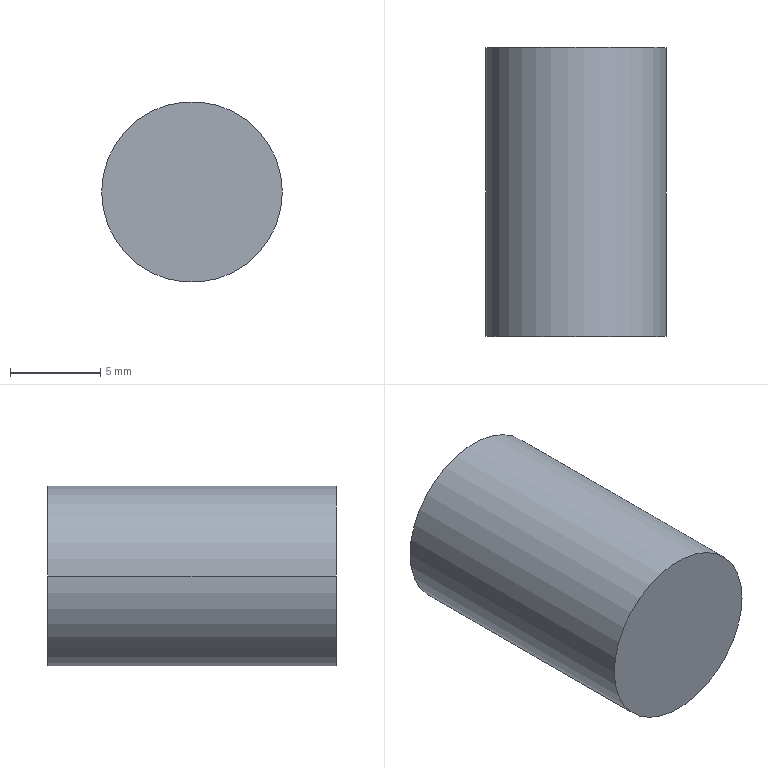Part | SolidWorks | features Chamfer 1, ICE 1, Revolution 1 | 1 solid | 9 faces | box 10 x 16 x 10 mm | volume 971.407 mm3 | cylinder 4 | plane 3 | cone 2 | commonest cylinder face diameters 6 x2 10 x2
STEP:
#1=CARTESIAN_POINT('',(3.,-0.5,0.));
#2=VERTEX_POINT('',#1);
#3=CARTESIAN_POINT('',(-3.,-0.5,0.));
#4=VERTEX_POINT('',#3);
#5=CARTESIAN_POINT('',(0.,-0.5,0.));
#6=DIRECTION('',(0.,1.,0.));
#7=DIRECTION('',(-1.,0.,0.));
#8=AXIS2_PLACEMENT_3D('',#5,#6,#7);
#9=CIRCLE('',#8,3.);
#10=EDGE_CURVE('',#2,#4,#9,.T.);
#11=ORIENTED_EDGE('',*,*,#10,.F.);
#12=CARTESIAN_POINT('',(3.5,0.,0.));
#13=VERTEX_POINT('',#12);
#14=CARTESIAN_POINT('',(3.,-0.5,0.));
#15=DIRECTION('',(0.7071,0.7071,0.));
#16=VECTOR('',#15,1000.);
#17=LINE('',#14,#16);
#18=EDGE_CURVE('',#2,#13,#17,.T.);
#19=ORIENTED_EDGE('',*,*,#18,.T.);
#20=CARTESIAN_POINT('',(-3.5,0.,0.));
#21=VERTEX_POINT('',#20);
#22=CARTESIAN_POINT('',(0.,0.,0.));
#23=DIRECTION('',(0.,-1.,0.));
#24=DIRECTION('',(-1.,0.,0.));
#25=AXIS2_PLACEMENT_3D('',#22,#23,#24);
#26=CIRCLE('',#25,3.5);
#27=EDGE_CURVE('',#21,#13,#26,.T.);
#28=ORIENTED_EDGE('',*,*,#27,.F.);
#29=CARTESIAN_POINT('',(-3.,-0.5,0.));
#30=DIRECTION('',(-0.7071,0.7071,0.));
#31=VECTOR('',#30,1000.);
#32=LINE('',#29,#31);
#33=EDGE_CURVE('',#4,#21,#32,.T.);
#34=ORIENTED_EDGE('',*,*,#33,.F.);
#35=EDGE_LOOP('',(#11,#19,#28,#34));
#36=FACE_OUTER_BOUND('',#35,.T.);
#37=CARTESIAN_POINT('',(0.,-0.5,0.));
#38=DIRECTION('',(0.,1.,0.));
#39=DIRECTION('',(-1.,0.,0.));
#40=AXIS2_PLACEMENT_3D('',#37,#38,#39);
#41=CONICAL_SURFACE('',#40,3.,0.7854);
#42=ADVANCED_FACE('',(#36),#41,.F.);
#43=CARTESIAN_POINT('',(3.,-10.,0.));
#44=VERTEX_POINT('',#43);
#45=CARTESIAN_POINT('',(-3.,-10.,0.));
#46=VERTEX_POINT('',#45);
#47=CARTESIAN_POINT('',(0.,-10.,0.));
#48=DIRECTION('',(0.,1.,0.));
#49=DIRECTION('',(-1.,0.,0.));
#50=AXIS2_PLACEMENT_3D('',#47,#48,#49);
#51=CIRCLE('',#50,3.);
#52=EDGE_CURVE('',#44,#46,#51,.T.);
#53=ORIENTED_EDGE('',*,*,#52,.F.);
#54=CARTESIAN_POINT('',(3.,-10.,0.));
#55=DIRECTION('',(0.,1.,0.));
#56=VECTOR('',#55,1000.);
#57=LINE('',#54,#56);
#58=EDGE_CURVE('',#44,#2,#57,.T.);
#59=ORIENTED_EDGE('',*,*,#58,.T.);
#60=ORIENTED_EDGE('',*,*,#10,.T.);
#61=CARTESIAN_POINT('',(-3.,-10.,0.));
#62=DIRECTION('',(0.,1.,0.));
#63=VECTOR('',#62,1000.);
#64=LINE('',#61,#63);
#65=EDGE_CURVE('',#46,#4,#64,.T.);
#66=ORIENTED_EDGE('',*,*,#65,.F.);
#67=EDGE_LOOP('',(#53,#59,#60,#66));
#68=FACE_OUTER_BOUND('',#67,.T.);
#69=CARTESIAN_POINT('',(0.,-10.,0.));
#70=DIRECTION('',(0.,1.,0.));
#71=DIRECTION('',(-1.,0.,0.));
#72=AXIS2_PLACEMENT_3D('',#69,#70,#71);
#73=CYLINDRICAL_SURFACE('',#72,3.);
#74=ADVANCED_FACE('',(#68),#73,.F.);
#75=CARTESIAN_POINT('',(5.,0.,0.));
#76=VERTEX_POINT('',#75);
#77=CARTESIAN_POINT('',(-5.,0.,0.));
#78=VERTEX_POINT('',#77);
#79=CARTESIAN_POINT('',(0.,0.,0.));
#80=DIRECTION('',(0.,-1.,0.));
#81=DIRECTION('',(1.,0.,0.));
#82=AXIS2_PLACEMENT_3D('',#79,#80,#81);
#83=CIRCLE('',#82,5.);
#84=EDGE_CURVE('',#76,#78,#83,.T.);
#85=ORIENTED_EDGE('',*,*,#84,.T.);
#86=CARTESIAN_POINT('',(-5.,-16.,0.));
#87=VERTEX_POINT('',#86);
#88=CARTESIAN_POINT('',(-5.,-264.304,0.));
#89=DIRECTION('',(0.,-1.,0.));
#90=VECTOR('',#89,1000.);
#91=LINE('',#88,#90);
#92=EDGE_CURVE('',#78,#87,#91,.T.);
#93=ORIENTED_EDGE('',*,*,#92,.T.);
#94=CARTESIAN_POINT('',(5.,-16.,0.));
#95=VERTEX_POINT('',#94);
#96=CARTESIAN_POINT('',(0.,-16.,0.));
#97=DIRECTION('',(0.,-1.,0.));
#98=DIRECTION('',(1.,0.,0.));
#99=AXIS2_PLACEMENT_3D('',#96,#97,#98);
#100=CIRCLE('',#99,5.);
#101=EDGE_CURVE('',#95,#87,#100,.T.);
#102=ORIENTED_EDGE('',*,*,#101,.F.);
#103=CARTESIAN_POINT('',(5.,-264.304,0.));
#104=DIRECTION('',(0.,-1.,0.));
#105=VECTOR('',#104,1000.);
#106=LINE('',#103,#105);
#107=EDGE_CURVE('',#76,#95,#106,.T.);
#108=ORIENTED_EDGE('',*,*,#107,.F.);
#109=EDGE_LOOP('',(#85,#93,#102,#108));
#110=FACE_OUTER_BOUND('',#109,.T.);
#111=CARTESIAN_POINT('',(0.,-264.304,0.));
#112=DIRECTION('',(0.,-1.,0.));
#113=DIRECTION('',(1.,0.,0.));
#114=AXIS2_PLACEMENT_3D('',#111,#112,#113);
#115=CYLINDRICAL_SURFACE('',#114,5.);
#116=ADVANCED_FACE('',(#110),#115,.T.);
#117=ORIENTED_EDGE('',*,*,#27,.T.);
#118=CARTESIAN_POINT('',(0.,0.,0.));
#119=DIRECTION('',(0.,-1.,0.));
#120=DIRECTION('',(-1.,0.,0.));
#121=AXIS2_PLACEMENT_3D('',#118,#119,#120);
#122=CIRCLE('',#121,3.5);
#123=EDGE_CURVE('',#13,#21,#122,.T.);
#124=ORIENTED_EDGE('',*,*,#123,.T.);
#125=EDGE_LOOP('',(#117,#124));
#126=FACE_BOUND('',#125,.T.);
#127=ORIENTED_EDGE('',*,*,#84,.F.);
#128=CARTESIAN_POINT('',(0.,0.,0.));
#129=DIRECTION('',(0.,-1.,0.));
#130=DIRECTION('',(1.,0.,0.));
#131=AXIS2_PLACEMENT_3D('',#128,#129,#130);
#132=CIRCLE('',#131,5.);
#133=EDGE_CURVE('',#78,#76,#132,.T.);
#134=ORIENTED_EDGE('',*,*,#133,.F.);
#135=EDGE_LOOP('',(#127,#134));
#136=FACE_OUTER_BOUND('',#135,.T.);
#137=CARTESIAN_POINT('',(0.,0.,0.));
#138=DIRECTION('',(0.,1.,0.));
#139=DIRECTION('',(-1.,0.,0.));
#140=AXIS2_PLACEMENT_3D('',#137,#138,#139);
#141=PLANE('',#140);
#142=ADVANCED_FACE('',(#126,#136),#141,.T.);
#143=ORIENTED_EDGE('',*,*,#92,.F.);
#144=ORIENTED_EDGE('',*,*,#133,.T.);
#145=ORIENTED_EDGE('',*,*,#107,.T.);
#146=CARTESIAN_POINT('',(0.,-16.,0.));
#147=DIRECTION('',(0.,-1.,0.));
#148=DIRECTION('',(1.,0.,0.));
#149=AXIS2_PLACEMENT_3D('',#146,#147,#148);
#150=CIRCLE('',#149,5.);
#151=EDGE_CURVE('',#87,#95,#150,.T.);
#152=ORIENTED_EDGE('',*,*,#151,.F.);
#153=EDGE_LOOP('',(#143,#144,#145,#152));
#154=FACE_OUTER_BOUND('',#153,.T.);
#155=CARTESIAN_POINT('',(0.,-264.304,0.));
#156=DIRECTION('',(0.,-1.,0.));
#157=DIRECTION('',(1.,0.,0.));
#158=AXIS2_PLACEMENT_3D('',#155,#156,#157);
#159=CYLINDRICAL_SURFACE('',#158,5.);
#160=ADVANCED_FACE('',(#154),#159,.T.);
#161=ORIENTED_EDGE('',*,*,#101,.T.);
#162=ORIENTED_EDGE('',*,*,#151,.T.);
#163=EDGE_LOOP('',(#161,#162));
#164=FACE_OUTER_BOUND('',#163,.T.);
#165=CARTESIAN_POINT('',(5.,-16.,0.));
#166=DIRECTION('',(0.,-1.,0.));
#167=DIRECTION('',(1.,0.,0.));
#168=AXIS2_PLACEMENT_3D('',#165,#166,#167);
#169=PLANE('',#168);
#170=ADVANCED_FACE('',(#164),#169,.T.);
#171=ORIENTED_EDGE('',*,*,#58,.F.);
#172=CARTESIAN_POINT('',(0.,-10.,0.));
#173=DIRECTION('',(0.,1.,0.));
#174=DIRECTION('',(-1.,0.,0.));
#175=AXIS2_PLACEMENT_3D('',#172,#173,#174);
#176=CIRCLE('',#175,3.);
#177=EDGE_CURVE('',#46,#44,#176,.T.);
#178=ORIENTED_EDGE('',*,*,#177,.F.);
#179=ORIENTED_EDGE('',*,*,#65,.T.);
#180=CARTESIAN_POINT('',(0.,-0.5,0.));
#181=DIRECTION('',(0.,1.,0.));
#182=DIRECTION('',(-1.,0.,0.));
#183=AXIS2_PLACEMENT_3D('',#180,#181,#182);
#184=CIRCLE('',#183,3.);
#185=EDGE_CURVE('',#4,#2,#184,.T.);
#186=ORIENTED_EDGE('',*,*,#185,.T.);
#187=EDGE_LOOP('',(#171,#178,#179,#186));
#188=FACE_OUTER_BOUND('',#187,.T.);
#189=CARTESIAN_POINT('',(0.,-10.,0.));
#190=DIRECTION('',(0.,1.,0.));
#191=DIRECTION('',(-1.,0.,0.));
#192=AXIS2_PLACEMENT_3D('',#189,#190,#191);
#193=CYLINDRICAL_SURFACE('',#192,3.);
#194=ADVANCED_FACE('',(#188),#193,.F.);
#195=ORIENTED_EDGE('',*,*,#177,.T.);
#196=ORIENTED_EDGE('',*,*,#52,.T.);
#197=EDGE_LOOP('',(#195,#196));
#198=FACE_OUTER_BOUND('',#197,.T.);
#199=CARTESIAN_POINT('',(0.,-10.,0.));
#200=DIRECTION('',(0.,1.,0.));
#201=DIRECTION('',(-1.,0.,0.));
#202=AXIS2_PLACEMENT_3D('',#199,#200,#201);
#203=PLANE('',#202);
#204=ADVANCED_FACE('',(#198),#203,.T.);
#205=ORIENTED_EDGE('',*,*,#18,.F.);
#206=ORIENTED_EDGE('',*,*,#185,.F.);
#207=ORIENTED_EDGE('',*,*,#33,.T.);
#208=ORIENTED_EDGE('',*,*,#123,.F.);
#209=EDGE_LOOP('',(#205,#206,#207,#208));
#210=FACE_OUTER_BOUND('',#209,.T.);
#211=CARTESIAN_POINT('',(0.,-0.5,0.));
#212=DIRECTION('',(0.,1.,0.));
#213=DIRECTION('',(-1.,0.,0.));
#214=AXIS2_PLACEMENT_3D('',#211,#212,#213);
#215=CONICAL_SURFACE('',#214,3.,0.7854);
#216=ADVANCED_FACE('',(#210),#215,.F.);
#217=CLOSED_SHELL('',(#42,#74,#116,#142,#160,#170,#194,#204,#216));
#218=MANIFOLD_SOLID_BREP('',#217);
#219=CARTESIAN_POINT('',(0.,0.,0.));
#220=DIRECTION('',(0.,0.,1.));
#221=DIRECTION('',(1.,0.,0.));
#222=AXIS2_PLACEMENT_3D('',#219,#220,#221);
#223=(LENGTH_UNIT()NAMED_UNIT(*)SI_UNIT(.MILLI.,.METRE.));
#224=UNCERTAINTY_MEASURE_WITH_UNIT(LENGTH_MEASURE(0.00001),#223,'','');
#225=(NAMED_UNIT(*)PLANE_ANGLE_UNIT()SI_UNIT($,.RADIAN.));
#226=(NAMED_UNIT(*)SI_UNIT($,.STERADIAN.)SOLID_ANGLE_UNIT());
#227=(GEOMETRIC_REPRESENTATION_CONTEXT(3)GLOBAL_UNCERTAINTY_ASSIGNED_CONTEXT((#224))GLOBAL_UNIT_ASSIGNED_CONTEXT((#223,#225,#226))REPRESENTATION_CONTEXT('',''));
#228=ADVANCED_BREP_SHAPE_REPRESENTATION('',(#218,#222),#227);